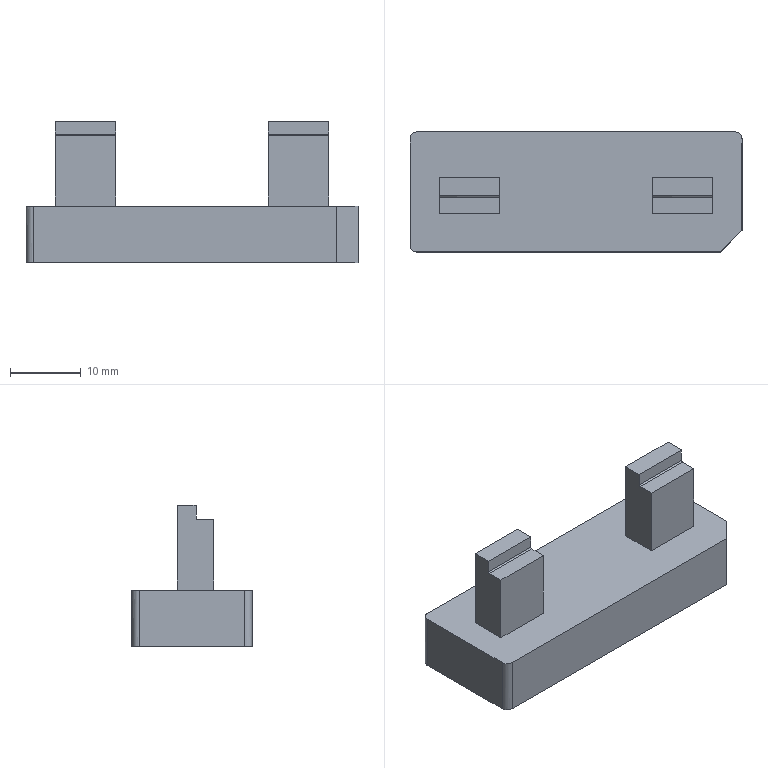NC program | PowerMill | posted by the shop | part box 47 x 17 x 19.985 mm
Lines 1 to 1597 of 62704:
%
G40 G49 G17 G80
( TOOL ID   D10C_1_1_1 )
( TOOL DIA. 10. TIP RAD 0 LENGTH 75.44 )
( Z = -.065 )
T1 M6
T2
G91 G28 Z0
G0 G90 G54
M08
S8000 M3
G0 X0 Y0 M8
G43 Z10.2 H1
X31.28 Y11.28
Z1.135
G1 Z-.065 F6000
X26.28 F10000
X-26.28
Y5.64
X26.28
Y0
X-26.28
Y-5.64
X26.28
Y-11.28
X-26.28
X-31.28
G0 Z10.2
X0 Y0
Z9.885
X-32.38 Y-5.333
Z.691
G1 Z-.509 F6000
X-31.853 F10000
G3 X-27.105 Y-.585 I0 J4.747
G1 Y10.28
G2 X-26.105 Y11.28 I1. J0
G1 X26.105
G2 X27.105 Y10.28 I0 J-1.
G1 Y2.243
X24.596 Y2.127
X24.605 Y1.934
Y-.387
X24.574 Y-1.16
X24.43 Y-1.934
X24.16 Y-2.707
X23.976 Y-3.084
X23.74 Y-3.48
X23.203 Y-4.168
X22.429 Y-4.856
X22.178 Y-5.027
X21.656 Y-5.322
X20.883 Y-5.63
X20.144 Y-5.801
X19.336 Y-5.865
X10.828
X10.055 Y-5.808
X9.281 Y-5.634
X8.508 Y-5.329
X7.972 Y-5.027
X7.734 Y-4.866
X7.028 Y-4.254
X6.41 Y-3.48
X6.187 Y-3.109
X6.165 Y-3.063
X.373 Y-4.753
X.381 Y-4.793
X.384 Y-4.833
G2 X-.192 Y-4.833 I-.288 J0
X.373 Y-4.753 I.288 J0
G1 X6.165 Y-3.063
X5.99 Y-2.707
X5.72 Y-1.934
X5.576 Y-1.16
X5.545 Y-.387
Y1.934
X5.581 Y2.707
X5.731 Y3.48
X.004 Y5.269
X.002 Y5.263
X0 Y5.258
X-.007 Y5.28
X.007
X.005 Y5.274
X.004 Y5.269
X5.731 Y3.48
X6.008 Y4.254
X6.187 Y4.616
X6.436 Y5.027
X6.961 Y5.69
X7.734 Y6.373
X8.034 Y6.574
X8.508 Y6.837
X9.281 Y7.142
X10.055 Y7.316
X10.828 Y7.372
X19.336
X20.109 Y7.314
X20.883 Y7.137
X21.656 Y6.83
X22.116 Y6.574
X22.429 Y6.363
X23.083 Y5.801
X23.714 Y5.027
X23.976 Y4.591
X24.142 Y4.254
X24.419 Y3.48
X24.569 Y2.707
X24.596 Y2.127
X27.105 Y2.243
Y-10.28
G2 X26.105 Y-11.28 I-1. J0
G1 X-26.105
G2 X-27.105 Y-10.28 I0 J1.
G1 Y-.585
X-24.601 Y-.483
X-24.605 Y-.387
Y1.934
X-24.569 Y2.707
X-24.419 Y3.48
X-24.142 Y4.254
X-23.976 Y4.592
X-23.714 Y5.027
X-23.203 Y5.676
X-22.429 Y6.364
X-22.117 Y6.574
X-21.656 Y6.83
X-20.883 Y7.138
X-20.109 Y7.314
X-19.336 Y7.373
X-10.828
X-10.055 Y7.316
X-9.281 Y7.142
X-8.508 Y6.837
X-8.033 Y6.574
X-7.734 Y6.374
X-7.066 Y5.801
X-6.436 Y5.027
X-6.187 Y4.617
X-6.008 Y4.254
X-5.731 Y3.48
X-5.581 Y2.707
X-5.545 Y1.934
Y-.387
X-5.577 Y-1.16
X-5.72 Y-1.934
X-5.99 Y-2.707
X-6.187 Y-3.108
X-6.41 Y-3.48
X-6.961 Y-4.182
X-7.734 Y-4.865
X-7.972 Y-5.027
X-8.508 Y-5.329
X-9.281 Y-5.634
X-10.008 Y-5.801
X-10.828 Y-5.864
X-19.336
X-20.109 Y-5.806
X-20.883 Y-5.629
X-21.656 Y-5.322
X-22.178 Y-5.027
X-22.429 Y-4.855
X-23.121 Y-4.254
X-23.74 Y-3.48
X-23.976 Y-3.083
X-24.159 Y-2.707
X-24.43 Y-1.934
X-24.573 Y-1.16
X-24.601 Y-.483
X-27.105 Y-.585
G0 Z3.297
G1 X-32.38 Y-5.333
G0 Z.297
G1 Z-.903 F6000
X-31.853 F10000
G3 X-27.105 Y-.585 I0 J4.747
G1 X-24.601 Y-.483
X-24.605 Y-.387
Y1.934
X-24.569 Y2.707
X-24.419 Y3.48
X-24.142 Y4.254
X-23.976 Y4.592
X-23.714 Y5.027
X-23.203 Y5.676
X-22.429 Y6.364
X-22.117 Y6.574
X-21.656 Y6.83
X-20.883 Y7.138
X-20.109 Y7.314
X-19.336 Y7.373
X-10.828
X-10.055 Y7.316
X-9.281 Y7.142
X-8.508 Y6.837
X-8.033 Y6.574
X-7.734 Y6.374
X-7.066 Y5.801
X-6.436 Y5.027
X-6.187 Y4.617
X-6.008 Y4.254
X-5.731 Y3.48
X-5.581 Y2.707
X-5.545 Y1.934
Y-.387
X-5.577 Y-1.16
X-5.72 Y-1.934
X-5.99 Y-2.707
X-6.187 Y-3.108
X-6.41 Y-3.48
X-6.961 Y-4.182
X-7.734 Y-4.865
X-7.972 Y-5.027
X-8.508 Y-5.329
X-9.281 Y-5.634
X-10.008 Y-5.801
X-10.828 Y-5.864
X-19.336
X-20.109 Y-5.806
X-20.883 Y-5.629
X-21.656 Y-5.322
X-22.178 Y-5.027
X-22.429 Y-4.855
X-23.121 Y-4.254
X-23.74 Y-3.48
X-23.976 Y-3.083
X-24.159 Y-2.707
X-24.43 Y-1.934
X-24.573 Y-1.16
X-24.601 Y-.483
X-27.105 Y-.585
Y10.28
G2 X-26.105 Y11.28 I1. J0
G1 X26.105
G2 X27.105 Y10.28 I0 J-1.
G1 Y2.243
X24.596 Y2.127
X24.605 Y1.934
Y-.387
X24.574 Y-1.16
X24.43 Y-1.934
X24.16 Y-2.707
X23.976 Y-3.084
X23.74 Y-3.48
X23.203 Y-4.168
X22.429 Y-4.856
X22.178 Y-5.027
X21.656 Y-5.322
X20.883 Y-5.63
X20.144 Y-5.801
X19.336 Y-5.865
X10.828
X10.055 Y-5.808
X9.281 Y-5.634
X8.508 Y-5.329
X7.972 Y-5.027
X7.734 Y-4.866
X7.028 Y-4.254
X6.41 Y-3.48
X6.187 Y-3.109
X6.165 Y-3.063
X.373 Y-4.753
X.381 Y-4.793
X.384 Y-4.833
G2 X-.192 Y-4.833 I-.288 J0
X.373 Y-4.753 I.288 J0
G1 X6.165 Y-3.063
X5.99 Y-2.707
X5.72 Y-1.934
X5.576 Y-1.16
X5.545 Y-.387
Y1.934
X5.581 Y2.707
X5.731 Y3.48
X.004 Y5.269
X.002 Y5.263
X0 Y5.258
X-.007 Y5.28
X.007
X.005 Y5.274
X.004 Y5.269
X5.731 Y3.48
X6.008 Y4.254
X6.187 Y4.616
X6.436 Y5.027
X6.961 Y5.69
X7.734 Y6.373
X8.034 Y6.574
X8.508 Y6.837
X9.281 Y7.142
X10.055 Y7.316
X10.828 Y7.372
X19.336
X20.109 Y7.314
X20.883 Y7.137
X21.656 Y6.83
X22.116 Y6.574
X22.429 Y6.363
X23.083 Y5.801
X23.714 Y5.027
X23.976 Y4.591
X24.142 Y4.254
X24.419 Y3.48
X24.569 Y2.707
X24.596 Y2.127
X27.105 Y2.243
Y-10.28
G2 X26.105 Y-11.28 I-1. J0
G1 X-26.105
G2 X-27.105 Y-10.28 I0 J1.
G1 Y-.585
G0 Z2.903
G1 X-32.38 Y-5.333
G0 Z-.097
G1 Z-1.297 F6000
X-31.853 F10000
G3 X-27.105 Y-.585 I0 J4.747
G1 X-24.601 Y-.483
X-24.605 Y-.387
Y1.934
X-24.569 Y2.707
X-24.419 Y3.48
X-24.142 Y4.254
X-23.976 Y4.592
X-23.714 Y5.027
X-23.203 Y5.676
X-22.429 Y6.364
X-22.117 Y6.574
X-21.656 Y6.83
X-20.883 Y7.138
X-20.109 Y7.314
X-19.336 Y7.373
X-10.828
X-10.055 Y7.316
X-9.281 Y7.142
X-8.508 Y6.837
X-8.033 Y6.574
X-7.734 Y6.374
X-7.066 Y5.801
X-6.436 Y5.027
X-6.187 Y4.617
X-6.008 Y4.254
X-5.731 Y3.48
X-5.581 Y2.707
X-5.545 Y1.934
Y-.387
X-5.577 Y-1.16
X-5.72 Y-1.934
X-5.99 Y-2.707
X-6.187 Y-3.108
X-6.41 Y-3.48
X-6.961 Y-4.182
X-7.734 Y-4.865
X-7.972 Y-5.027
X-8.508 Y-5.329
X-9.281 Y-5.634
X-10.008 Y-5.801
X-10.828 Y-5.864
X-19.336
X-20.109 Y-5.806
X-20.883 Y-5.629
X-21.656 Y-5.322
X-22.178 Y-5.027
X-22.429 Y-4.855
X-23.121 Y-4.254
X-23.74 Y-3.48
X-23.976 Y-3.083
X-24.16 Y-2.707
X-24.43 Y-1.934
X-24.573 Y-1.16
X-24.601 Y-.483
X-27.105 Y-.585
Y10.28
G2 X-26.105 Y11.28 I1. J0
G1 X26.105
G2 X27.105 Y10.28 I0 J-1.
G1 Y2.243
X24.596 Y2.127
X24.605 Y1.934
Y-.387
X24.574 Y-1.16
X24.43 Y-1.934
X24.16 Y-2.707
X23.976 Y-3.084
X23.74 Y-3.48
X23.203 Y-4.168
X22.429 Y-4.856
X22.178 Y-5.027
X21.656 Y-5.322
X20.883 Y-5.63
X20.144 Y-5.801
X19.336 Y-5.865
X10.828
X10.055 Y-5.808
X9.281 Y-5.634
X8.508 Y-5.329
X7.972 Y-5.027
X7.734 Y-4.866
X7.028 Y-4.254
X6.41 Y-3.48
X6.187 Y-3.109
X6.165 Y-3.063
X.373 Y-4.753
X.381 Y-4.793
X.384 Y-4.833
G2 X-.192 Y-4.833 I-.288 J0
X.373 Y-4.753 I.288 J0
G1 X6.165 Y-3.063
X5.99 Y-2.707
X5.72 Y-1.934
X5.576 Y-1.16
X5.545 Y-.387
Y1.934
X5.581 Y2.707
X5.731 Y3.48
X.004 Y5.269
X.002 Y5.263
X0 Y5.258
X-.007 Y5.28
X.007
X.005 Y5.274
X.004 Y5.269
X5.731 Y3.48
X6.008 Y4.254
X6.187 Y4.616
X6.436 Y5.027
X6.961 Y5.69
X7.734 Y6.373
X8.034 Y6.574
X8.508 Y6.837
X9.281 Y7.142
X10.055 Y7.316
X10.828 Y7.372
X19.336
X20.109 Y7.314
X20.883 Y7.137
X21.656 Y6.83
X22.116 Y6.574
X22.429 Y6.363
X23.083 Y5.801
X23.714 Y5.027
X23.976 Y4.591
X24.142 Y4.254
X24.419 Y3.48
X24.569 Y2.707
X24.596 Y2.127
X27.105 Y2.243
Y-10.28
G2 X26.105 Y-11.28 I-1. J0
G1 X-26.105
G2 X-27.105 Y-10.28 I0 J1.
G1 Y-.585
G0 Z2.509
G1 X-32.38 Y-5.333
G0 Z-.491
G1 Z-1.691 F6000
X-31.853 F10000
G3 X-27.105 Y-.585 I0 J4.747
G1 X-24.601 Y-.483
X-24.605 Y-.387
Y1.934
X-24.569 Y2.707
X-24.419 Y3.48
X-24.142 Y4.254
X-23.976 Y4.592
X-23.714 Y5.027
X-23.203 Y5.676
X-22.429 Y6.364
X-22.117 Y6.574
X-21.656 Y6.83
X-20.883 Y7.138
X-20.109 Y7.314
X-19.336 Y7.373
X-10.828
X-10.055 Y7.316
X-9.281 Y7.142
X-8.508 Y6.837
X-8.033 Y6.574
X-7.734 Y6.374
X-7.066 Y5.801
X-6.436 Y5.027
X-6.187 Y4.617
X-6.008 Y4.254
X-5.731 Y3.48
X-5.581 Y2.707
X-5.545 Y1.934
Y-.387
X-5.576 Y-1.16
X-5.72 Y-1.934
X-5.99 Y-2.707
X-6.187 Y-3.108
X-6.41 Y-3.48
X-6.961 Y-4.182
X-7.734 Y-4.865
X-7.972 Y-5.027
X-8.508 Y-5.329
X-9.281 Y-5.634
X-10.008 Y-5.801
X-10.828 Y-5.864
X-19.336
X-20.109 Y-5.806
X-20.883 Y-5.629
X-21.656 Y-5.322
X-22.178 Y-5.027
X-22.429 Y-4.855
X-23.121 Y-4.254
X-23.74 Y-3.48
X-23.976 Y-3.083
X-24.16 Y-2.707
X-24.43 Y-1.934
X-24.574 Y-1.16
X-24.601 Y-.483
X-27.105 Y-.585
Y10.28
G2 X-26.105 Y11.28 I1. J0
G1 X26.105
G2 X27.105 Y10.28 I0 J-1.
G1 Y2.243
X24.596 Y2.127
X24.605 Y1.934
Y-.387
X24.574 Y-1.16
X24.43 Y-1.934
X24.16 Y-2.707
X23.976 Y-3.084
X23.74 Y-3.48
X23.203 Y-4.168
X22.429 Y-4.856
X22.178 Y-5.027
X21.656 Y-5.322
X20.883 Y-5.63
X20.144 Y-5.801
X19.336 Y-5.865
X10.828
X10.055 Y-5.808
X9.281 Y-5.634
X8.508 Y-5.329
X7.972 Y-5.027
X7.734 Y-4.866
X7.028 Y-4.254
X6.41 Y-3.48
X6.187 Y-3.109
X6.165 Y-3.063
X.373 Y-4.753
X.381 Y-4.793
X.384 Y-4.833
G2 X-.192 Y-4.833 I-.288 J0
X.373 Y-4.753 I.288 J0
G1 X6.165 Y-3.063
X5.99 Y-2.707
X5.72 Y-1.934
X5.576 Y-1.16
X5.545 Y-.387
Y1.934
X5.581 Y2.707
X5.731 Y3.48
X.004 Y5.269
X.002 Y5.263
X0 Y5.258
X-.007 Y5.28
X.007
X.005 Y5.274
X.004 Y5.269
X5.731 Y3.48
X6.008 Y4.254
X6.187 Y4.616
X6.436 Y5.027
X6.961 Y5.69
X7.734 Y6.373
X8.034 Y6.574
X8.508 Y6.837
X9.281 Y7.142
X10.055 Y7.316
X10.828 Y7.372
X19.336
X20.109 Y7.314
X20.883 Y7.137
X21.656 Y6.83
X22.116 Y6.574
X22.429 Y6.363
X23.083 Y5.801
X23.714 Y5.027
X23.976 Y4.591
X24.142 Y4.254
X24.419 Y3.48
X24.569 Y2.707
X24.596 Y2.127
X27.105 Y2.243
Y-10.28
G2 X26.105 Y-11.28 I-1. J0
G1 X-26.105
G2 X-27.105 Y-10.28 I0 J1.
G1 Y-.585
G0 Z2.115
G1 X-32.38 Y-5.333
G0 Z-.885
G1 Z-2.085 F6000
X-31.853 F10000
G3 X-27.105 Y-.585 I0 J4.747
G1 Y-.387
X-24.605
Y1.934
X-24.569 Y2.707
X-24.419 Y3.48
X-24.142 Y4.254
X-23.976 Y4.592
X-23.714 Y5.027
X-23.203 Y5.676
X-22.429 Y6.364
X-22.117 Y6.574
X-21.656 Y6.83
X-20.883 Y7.138
X-20.109 Y7.314
X-19.336 Y7.373
X-10.828
X-10.055 Y7.316
X-9.281 Y7.142
X-8.508 Y6.837
X-8.033 Y6.574
X-7.734 Y6.374
X-7.066 Y5.801
X-6.436 Y5.027
X-6.187 Y4.617
X-6.008 Y4.254
X-5.731 Y3.48
X-5.581 Y2.707
X-5.545 Y1.934
Y-.387
X-5.573 Y-1.16
X-5.688 Y-1.934
X-5.976 Y-2.707
X-6.187 Y-3.145
X-6.384 Y-3.48
X-6.961 Y-4.224
X-7.734 Y-4.91
X-8.508 Y-5.376
X-9.281 Y-5.683
X-9.738 Y-5.801
X-10.055 Y-5.858
X-10.828 Y-5.914
X-19.336
X-20.109 Y-5.855
X-20.883 Y-5.679
X-21.656 Y-5.37
X-22.429 Y-4.901
X-23.164 Y-4.254
X-23.775 Y-3.48
X-24.175 Y-2.707
X-24.438 Y-1.934
X-24.58 Y-1.16
X-24.605 Y-.387
X-27.105
Y10.28
G2 X-26.105 Y11.28 I1. J0
G1 X26.105
G2 X27.105 Y10.28 I0 J-1.
G1 Y2.243
X24.596 Y2.127
X24.605 Y1.934
Y-.387
X24.58 Y-1.16
X24.438 Y-1.934
X24.175 Y-2.707
X23.976 Y-3.122
X23.764 Y-3.48
X23.203 Y-4.21
X22.429 Y-4.901
X22.254 Y-5.027
X21.656 Y-5.37
X20.883 Y-5.679
X20.423 Y-5.801
X20.109 Y-5.856
X19.336 Y-5.915
X10.828
X10.055 Y-5.859
X9.281 Y-5.683
X8.508 Y-5.377
X7.896 Y-5.027
X7.734 Y-4.911
X6.986 Y-4.254
X6.384 Y-3.48
X6.187 Y-3.146
X6.154 Y-3.078
X.315 Y-4.781
X.322 Y-4.816
X.325 Y-4.851
G2 X-.18 Y-4.851 I-.252 J0
X.315 Y-4.781 I.252 J0
G1 X6.154 Y-3.078
X5.97 Y-2.707
X5.688 Y-1.934
X5.573 Y-1.16
X5.545 Y-.387
Y1.934
X5.581 Y2.707
X5.731 Y3.48
X.004 Y5.269
X.002 Y5.263
X0 Y5.258
X-.007 Y5.28
X.007
X.005 Y5.274
X.004 Y5.269
X5.731 Y3.48
X6.008 Y4.254
X6.187 Y4.616
X6.436 Y5.027
X6.961 Y5.69
X7.734 Y6.373
X8.034 Y6.574
X8.508 Y6.837
X9.281 Y7.142
X10.055 Y7.316
X10.828 Y7.372
X19.336
X20.109 Y7.314
X20.883 Y7.137
X21.656 Y6.83
X22.116 Y6.574
X22.429 Y6.363
X23.084 Y5.801
X23.714 Y5.027
X23.976 Y4.591
X24.142 Y4.254
X24.419 Y3.48
X24.569 Y2.707
X24.596 Y2.127
X27.105 Y2.243
Y-10.28
G2 X26.105 Y-11.28 I-1. J0
G1 X-26.105
G2 X-27.105 Y-10.28 I0 J1.
G1 Y-.585
G0 Z1.719
G1 X-32.38 Y-5.333
G0 Z-1.281
G1 Z-2.481 F6000
X-31.853 F10000
G3 X-27.105 Y-.585 I0 J4.747
G1 Y10.28
G2 X-26.105 Y11.28 I1. J0
G1 X26.105
G2 X27.105 Y10.28 I0 J-1.
G1 Y2.243
X24.596 Y2.127
X24.605 Y1.934
Y1.913
Y-.387
X24.598 Y-.592
X24.591 Y-3.48
X24.476 Y-4.254
X24.238 Y-5.027
X23.857 Y-5.801
X23.294 Y-6.574
X22.451 Y-7.348
X21.656 Y-7.83
X20.935 Y-8.121
X20.109 Y-8.314
X19.336 Y-8.372
X10.828
X10.055 Y-8.316
X9.281 Y-8.142
X8.508 Y-7.837
X7.734 Y-7.373
X6.961 Y-6.69
X6.293 Y-5.801
X5.912 Y-5.027
X5.674 Y-4.254
X5.559 Y-3.48
X5.552 Y-.571
X5.549 Y-.497
X.081
Y-3.098
G3 X.275 Y-5.117 I10.557 J0
G1 X.325 Y-5.369
X.375 Y-5.597
G2 X.2 Y-5.815 I-.175 J-.039
G1 X-.2
G2 X-.375 Y-5.597 I0 J.179
G1 X-.348 Y-5.473
G3 X-.027 Y-2.387 I-13.16 J2.925
G1 X-.082 Y2.241
G3 X-.358 Y4.506 I-10.471 J-.124
G1 X-.401 Y4.69
X-.511 Y5.097
X-.646 Y5.497
X-.681 Y5.589
G2 X-.525 Y5.815 I.156 J.059
G1 X.525
G2 X.681 Y5.589 I0 J-.167
G1 X.647 Y5.497
X.512 Y5.101
X.403 Y4.696
X.362 Y4.522
G3 X.081 Y2.104 I10.268 J-2.418
G1 Y-.497
X5.549
X5.545 Y-.387
Y1.914
Y1.934
X5.581 Y2.707
X5.731 Y3.48
X6.008 Y4.254
X6.187 Y4.616
X6.436 Y5.027
X6.961 Y5.69
X7.734 Y6.373
X8.034 Y6.574
X8.508 Y6.837
X9.281 Y7.142
X10.055 Y7.316
X10.828 Y7.372
X19.336
X20.109 Y7.314
X20.883 Y7.137
X21.656 Y6.83
X22.116 Y6.574
X22.429 Y6.363
X23.084 Y5.801
X23.714 Y5.027
X23.976 Y4.591
X24.142 Y4.254
X24.419 Y3.48
X24.569 Y2.707
X24.596 Y2.127
X27.105 Y2.243
Y-10.28
G2 X26.105 Y-11.28 I-1. J0
G1 X-26.105
G2 X-27.105 Y-10.28 I0 J1.
G1 Y-3.487
X-24.591 Y-3.48
X-24.598 Y-.591
X-24.605 Y-.387
Y1.913
Y1.934
X-24.569 Y2.707
X-24.419 Y3.48
X-24.142 Y4.254
X-23.976 Y4.592
X-23.714 Y5.027
X-23.203 Y5.676
X-22.429 Y6.364
X-22.117 Y6.574
X-21.656 Y6.83
X-20.883 Y7.138
X-20.109 Y7.314
X-19.336 Y7.373
X-10.828
X-10.055 Y7.316
X-9.281 Y7.142
X-8.508 Y6.837
X-8.033 Y6.574
X-7.734 Y6.374
X-7.066 Y5.801
X-6.436 Y5.027
X-6.187 Y4.617
X-6.008 Y4.254
X-5.731 Y3.48
X-5.581 Y2.707
X-5.545 Y1.934
Y1.914
Y-.387
X-5.552 Y-.571
X-5.559 Y-3.48
X-5.674 Y-4.254
X-5.912 Y-5.027
X-6.293 Y-5.801
X-6.856 Y-6.574
X-7.7 Y-7.348
X-8.508 Y-7.836
X-9.216 Y-8.121
X-10.055 Y-8.315
X-10.828 Y-8.372
X-19.336
X-20.109 Y-8.313
X-20.883 Y-8.137
X-21.656 Y-7.83
X-22.45 Y-7.348
X-23.203 Y-6.675
X-23.857 Y-5.801
X-24.238 Y-5.027
X-24.476 Y-4.254
X-24.591 Y-3.48
X-27.105 Y-3.487
Y-.585
G0 Z1.322
G1 X-32.38 Y-5.333
G0 Z-1.678
G1 Z-2.878 F6000
X-31.853 F10000
G3 X-27.105 Y-.585 I0 J4.747
G1 Y10.28
G2 X-26.105 Y11.28 I1. J0
G1 X26.105
G2 X27.105 Y10.28 I0 J-1.
G1 Y2.243
X24.596 Y2.127
X24.605 Y1.934
Y1.894
Y-.387
X24.598 Y-.59
X24.591 Y-3.48
X24.476 Y-4.254
X24.238 Y-5.027
X23.857 Y-5.801
X23.294 Y-6.574
X22.451 Y-7.348
X21.656 Y-7.83
X20.935 Y-8.121
X20.109 Y-8.314
X19.336 Y-8.372
X10.828
X10.055 Y-8.316
X9.281 Y-8.142
X8.508 Y-7.837
X7.734 Y-7.373
X6.961 Y-6.69
X6.293 Y-5.801
X5.912 Y-5.027
X5.674 Y-4.254
X5.559 Y-3.48
X5.552 Y-.569
X5.549 Y-.497
X.081
Y-3.098
G3 X.276 Y-5.12 I10.562 J0
G1 X.325 Y-5.37
X.375 Y-5.597
G2 X.2 Y-5.815 I-.175 J-.039
G1 X-.2
G2 X-.375 Y-5.597 I0 J.179
G1 X-.347 Y-5.472
G3 X-.027 Y-2.383 I-13.169 J2.926
G1 X-.083 Y2.254
G3 X-.355 Y4.494 I-10.396 J-.126
G1 X-.4 Y4.685
X-.51 Y5.095
X-.646 Y5.497
X-.681 Y5.589
G2 X-.524 Y5.815 I.157 J.059
G1 X.525
G2 X.681 Y5.589 I0 J-.167
G1 X.647 Y5.497
X.512 Y5.101
X.403 Y4.698
X.362 Y4.525
G3 X.081 Y2.103 I10.273 J-2.421
G1 Y-.497
X5.549
X5.545 Y-.387
Y1.893
Y1.934
X5.581 Y2.707
X5.731 Y3.48
X6.008 Y4.254
X6.187 Y4.616
X6.436 Y5.027
X6.961 Y5.69
X7.734 Y6.373
X8.034 Y6.574
X8.508 Y6.837
X9.281 Y7.142
X10.055 Y7.316
X10.828 Y7.372
X19.336
X20.109 Y7.314
X20.883 Y7.137
X21.656 Y6.83
X22.116 Y6.574
X22.429 Y6.363
X23.084 Y5.801
X23.714 Y5.027
X23.976 Y4.591
X24.142 Y4.254
X24.419 Y3.48
X24.569 Y2.707
X24.596 Y2.127
X27.105 Y2.243
Y-10.28
G2 X26.105 Y-11.28 I-1. J0
G1 X-26.105
G2 X-27.105 Y-10.28 I0 J1.
G1 Y-3.487
X-24.591 Y-3.48
X-24.598 Y-.589
X-24.605 Y-.387
Y1.894
Y1.934
X-24.569 Y2.707
X-24.419 Y3.48
X-24.142 Y4.254
X-23.976 Y4.592
X-23.714 Y5.027
X-23.203 Y5.676
X-22.429 Y6.364
X-22.117 Y6.574
X-21.656 Y6.83
X-20.883 Y7.138
X-20.109 Y7.314
X-19.336 Y7.373
X-10.828
X-10.055 Y7.316
X-9.281 Y7.142
X-8.508 Y6.837
X-8.033 Y6.574
X-7.734 Y6.374
X-7.066 Y5.801
X-6.436 Y5.027
X-6.187 Y4.617
X-6.008 Y4.254
X-5.731 Y3.48
X-5.581 Y2.707
X-5.545 Y1.934
Y1.893
Y-.387
X-5.552 Y-.569
X-5.559 Y-3.48
X-5.674 Y-4.254
X-5.912 Y-5.027
X-6.293 Y-5.801
X-6.856 Y-6.574
X-7.7 Y-7.348
X-8.508 Y-7.836
X-9.216 Y-8.121
X-10.055 Y-8.315
X-10.828 Y-8.372
X-19.336
X-20.109 Y-8.313
X-20.883 Y-8.137
X-21.656 Y-7.83
X-22.45 Y-7.348
X-23.203 Y-6.675
X-23.857 Y-5.801
X-24.238 Y-5.027
X-24.476 Y-4.254
X-24.591 Y-3.48
X-27.105 Y-3.487
Y-.585
G0 Z.926
G1 X-32.38 Y-5.333
G0 Z-2.074
G1 Z-3.274 F6000
X-31.853 F10000
G3 X-27.105 Y-.585 I0 J4.747
G1 Y10.28
G2 X-26.105 Y11.28 I1. J0
G1 X26.105
G2 X27.105 Y10.28 I0 J-1.
G1 Y2.243
X24.596 Y2.127
X24.605 Y1.934
Y1.873
Y-.387
X24.598 Y-.588
X24.591 Y-3.48
X24.476 Y-4.254
X24.238 Y-5.027
X23.857 Y-5.801
X23.294 Y-6.574
X22.451 Y-7.348
X21.656 Y-7.83
X20.935 Y-8.121
X20.109 Y-8.314
X19.336 Y-8.372
X10.828
X10.055 Y-8.316
X9.281 Y-8.142
X8.508 Y-7.837
X7.734 Y-7.373
X6.961 Y-6.69
X6.293 Y-5.801
X5.912 Y-5.027
X5.674 Y-4.254
X5.559 Y-3.48
X5.552 Y-.568
X5.549 Y-.497
X.081
Y-3.097
G3 X.277 Y-5.123 I10.568 J0
G1 X.325 Y-5.37
X.375 Y-5.597
G2 X.2 Y-5.815 I-.175 J-.039
G1 X-.2
G2 X-.375 Y-5.597 I0 J.18
G1 X-.347 Y-5.471
G3 X-.027 Y-2.378 I-13.178 J2.927
G1 X-.084 Y2.266
G3 X-.353 Y4.483 I-10.328 J-.127
G1 X-.399 Y4.681
X-.509 Y5.093
X-.646 Y5.497
X-.681 Y5.589
G2 X-.524 Y5.815 I.157 J.059
G1 X.524
G2 X.681 Y5.589 I0 J-.167
G1 X.646 Y5.497
X.512 Y5.102
X.403 Y4.699
X.363 Y4.527
G3 X.081 Y2.103 I10.278 J-2.425
G1 Y-.497
X5.549
X5.545 Y-.387
Y1.873
Y1.934
X5.581 Y2.707
X5.731 Y3.48
X6.008 Y4.254
X6.187 Y4.616
X6.436 Y5.027
X6.961 Y5.69
X7.734 Y6.373
X8.034 Y6.574
X8.508 Y6.837
X9.281 Y7.142
X10.055 Y7.316
X10.828 Y7.372
X19.336
X20.109 Y7.314
X20.883 Y7.137
X21.656 Y6.83
X22.116 Y6.574
X22.429 Y6.363
X23.084 Y5.801
X23.714 Y5.027
X23.976 Y4.591
X24.142 Y4.254
X24.419 Y3.48
X24.569 Y2.707
X24.596 Y2.127
X27.105 Y2.243
Y-10.28
G2 X26.105 Y-11.28 I-1. J0
G1 X-26.105
G2 X-27.105 Y-10.28 I0 J1.
G1 Y-3.487
X-24.591 Y-3.48
X-24.598 Y-.587
X-24.605 Y-.387
Y1.873
Y1.934
X-24.569 Y2.707
X-24.419 Y3.48
X-24.142 Y4.254
X-23.976 Y4.592
X-23.714 Y5.027
X-23.203 Y5.676
X-22.429 Y6.364
X-22.117 Y6.574
X-21.656 Y6.83
X-20.883 Y7.138
X-20.109 Y7.314
X-19.336 Y7.373
X-10.828
X-10.055 Y7.316
X-9.281 Y7.142
X-8.508 Y6.837
X-8.033 Y6.574
X-7.734 Y6.374
X-7.066 Y5.801
X-6.436 Y5.027
X-6.187 Y4.617
X-6.008 Y4.254
X-5.731 Y3.48
X-5.581 Y2.707
X-5.545 Y1.934
Y1.873
Y-.387
X-5.552 Y-.568
X-5.559 Y-3.48
X-5.674 Y-4.254
X-5.912 Y-5.027
X-6.293 Y-5.801
X-6.856 Y-6.574
X-7.7 Y-7.348
X-8.508 Y-7.836
X-9.216 Y-8.121
X-10.055 Y-8.315
X-10.828 Y-8.372
X-19.336
X-20.109 Y-8.313
X-20.883 Y-8.137
X-21.656 Y-7.83
X-22.45 Y-7.348
X-23.203 Y-6.675
X-23.857 Y-5.801
X-24.238 Y-5.027
X-24.476 Y-4.254
X-24.591 Y-3.48
X-27.105 Y-3.487
Y-.585
G0 Z.53
G1 X-32.38 Y-5.333
G0 Z-2.47
G1 Z-3.67 F6000
X-31.853 F10000
G3 X-27.105 Y-.585 I0 J4.747
G1 Y10.28
G2 X-26.105 Y11.28 I1. J0
G1 X26.105
G2 X27.105 Y10.28 I0 J-1.
G1 Y2.243
X24.596 Y2.127
X24.605 Y1.934
Y1.853
Y-.387
X24.598 Y-.587
X24.591 Y-3.48
X24.476 Y-4.254
X24.238 Y-5.027
X23.857 Y-5.801
X23.294 Y-6.574
X22.451 Y-7.348
X21.656 Y-7.83
X20.935 Y-8.121
X20.109 Y-8.314
X19.336 Y-8.372
X10.828
X10.055 Y-8.316
X9.281 Y-8.142
X8.508 Y-7.837
X7.734 Y-7.373
X6.961 Y-6.69
X6.293 Y-5.801
X5.912 Y-5.027
X5.674 Y-4.254
X5.559 Y-3.48
X5.552 Y-.566
X5.549 Y-.497
X.081 Y-.498
Y-3.097
G3 X.277 Y-5.126 I10.574 J0
G1 X.325 Y-5.371
X.375 Y-5.596
G2 X.2 Y-5.815 I-.176 J-.039
G1 X-.2
G2 X-.375 Y-5.596 I0 J.18
G1 X-.347 Y-5.47
G3 X-.027 Y-2.374 I-13.187 J2.928
G1 X-.085 Y2.277
G3 X-.351 Y4.473 I-10.264 J-.128
G1 X-.398 Y4.678
X-.509 Y5.091
X-.646 Y5.497
X-.681 Y5.588
G2 X-.524 Y5.815 I.157 J.059
G1 X.524
G2 X.681 Y5.588 I0 J-.168
G1 X.646 Y5.497
X.512 Y5.102
X.404 Y4.7
X.363 Y4.53
G3 X.081 Y2.102 I10.283 J-2.428
G1 Y-.498
X5.549 Y-.497
X5.545 Y-.387
Y1.853
Y1.934
X5.581 Y2.707
X5.731 Y3.48
X6.008 Y4.254
X6.187 Y4.616
X6.436 Y5.027
X6.961 Y5.69
X7.734 Y6.373
X8.034 Y6.574
X8.508 Y6.837
X9.281 Y7.142
X10.055 Y7.316
X10.828 Y7.372
X19.336
X20.109 Y7.314
X20.883 Y7.137
X21.656 Y6.83
X22.116 Y6.574
X22.429 Y6.363
X23.084 Y5.801
X23.714 Y5.027
X23.976 Y4.591
X24.142 Y4.254
X24.419 Y3.48
X24.569 Y2.707
X24.596 Y2.127
X27.105 Y2.243
Y-10.28
G2 X26.105 Y-11.28 I-1. J0
G1 X-26.105
G2 X-27.105 Y-10.28 I0 J1.
G1 Y-3.487
X-24.591 Y-3.48
X-24.598 Y-.586
X-24.605 Y-.387
Y1.853
Y1.934
X-24.569 Y2.707
X-24.419 Y3.48
X-24.142 Y4.254
X-23.976 Y4.592
X-23.714 Y5.027
X-23.203 Y5.676
X-22.429 Y6.364
X-22.117 Y6.574
X-21.656 Y6.83
X-20.883 Y7.138
X-20.109 Y7.314
X-19.336 Y7.373
X-10.828
X-10.055 Y7.316
X-9.281 Y7.142
X-8.508 Y6.837
X-8.033 Y6.574
X-7.734 Y6.374
X-7.066 Y5.801
X-6.436 Y5.027
X-6.187 Y4.617
X-6.008 Y4.254
X-5.731 Y3.48
X-5.581 Y2.707
X-5.545 Y1.934
Y1.853
Y-.387
X-5.552 Y-.566
X-5.559 Y-3.48
X-5.674 Y-4.254
X-5.912 Y-5.027
X-6.293 Y-5.801
X-6.856 Y-6.574
X-7.7 Y-7.348
X-8.508 Y-7.836
X-9.216 Y-8.121
X-10.055 Y-8.315
X-10.828 Y-8.372
X-19.336
X-20.109 Y-8.313
X-20.883 Y-8.137
X-21.656 Y-7.83
X-22.45 Y-7.348
X-23.203 Y-6.675
X-23.857 Y-5.801
X-24.238 Y-5.027
X-24.476 Y-4.254
X-24.591 Y-3.48
X-27.105 Y-3.487
Y-.585
G0 Z.134
G1 X-32.38 Y-5.333
G0 Z-2.866
G1 Z-4.066 F6000
X-31.853 F10000
G3 X-27.105 Y-.585 I0 J4.747
G1 Y10.28
G2 X-26.105 Y11.28 I1. J0
G1 X26.105
G2 X27.105 Y10.28 I0 J-1.
G1 Y2.243
X24.596 Y2.127
X24.605 Y1.934
Y1.833
Y-.387
X24.598 Y-.585
X24.591 Y-3.48
X24.476 Y-4.254
X24.238 Y-5.027
X23.857 Y-5.801
X23.294 Y-6.574
X22.451 Y-7.348
X21.656 Y-7.83
X20.935 Y-8.121
X20.109 Y-8.314
X19.336 Y-8.372
X10.828
X10.055 Y-8.316
X9.281 Y-8.142
X8.508 Y-7.837
X7.734 Y-7.373
X6.961 Y-6.69
X6.293 Y-5.801
X5.912 Y-5.027
X5.674 Y-4.254
X5.559 Y-3.48
X5.552 Y-.564
X5.549 Y-.498
X.081
Y-3.097
G3 X.278 Y-5.128 I10.579 J0
G1 X.326 Y-5.371
X.375 Y-5.596
G2 X.199 Y-5.815 I-.176 J-.039
G1 X-.199
G2 X-.375 Y-5.596 I0 J.18
G1 X-.347 Y-5.469
G3 X-.027 Y-2.369 I-13.196 J2.929
G1 X-.086 Y2.287
G3 X-.349 Y4.464 I-10.204 J-.129
G1 X-.398 Y4.675
X-.508 Y5.09
X-.646 Y5.496
X-.681 Y5.588
G2 X-.524 Y5.815 I.157 J.059
G1 X.524
G2 X.681 Y5.588 I0 J-.168
G1 X.646 Y5.496
X.512 Y5.103
X.404 Y4.702
X.364 Y4.533
G3 X.081 Y2.101 I10.288 J-2.432
G1 Y-.498
X5.549
X5.545 Y-.387
Y1.833
Y1.934
X5.581 Y2.707
X5.731 Y3.48
X6.008 Y4.254
X6.187 Y4.616
X6.436 Y5.027
X6.961 Y5.69
X7.734 Y6.373
X8.034 Y6.574
X8.508 Y6.837
X9.281 Y7.142
X10.055 Y7.316
X10.828 Y7.372
X19.336
X20.109 Y7.314
X20.883 Y7.137
X21.656 Y6.83
X22.116 Y6.574
X22.429 Y6.363
X23.084 Y5.801
X23.714 Y5.027
X23.976 Y4.591
X24.142 Y4.254
X24.419 Y3.48
X24.569 Y2.707
X24.596 Y2.127
X27.105 Y2.243
Y-10.28
G2 X26.105 Y-11.28 I-1. J0
G1 X-26.105
G2 X-27.105 Y-10.28 I0 J1.
G1 Y-3.487
X-24.591 Y-3.48
X-24.598 Y-.584
X-24.605 Y-.387
Y1.833
Y1.934
X-24.569 Y2.707
X-24.419 Y3.48
X-24.142 Y4.254
X-23.976 Y4.592
X-23.714 Y5.027
X-23.203 Y5.676
X-22.429 Y6.364
X-22.117 Y6.574
X-21.656 Y6.83
X-20.883 Y7.138
X-20.109 Y7.314
X-19.336 Y7.373
X-10.828
X-10.055 Y7.316
X-9.281 Y7.142
X-8.508 Y6.837
X-8.033 Y6.574
X-7.734 Y6.374
X-7.066 Y5.801
X-6.436 Y5.027
X-6.187 Y4.617
X-6.008 Y4.254
X-5.731 Y3.48
X-5.581 Y2.707
X-5.545 Y1.934
Y1.833
Y-.387
X-5.552 Y-.564
X-5.559 Y-3.48
X-5.674 Y-4.254
X-5.912 Y-5.027
X-6.293 Y-5.801
X-6.856 Y-6.574
X-7.7 Y-7.348
X-8.508 Y-7.836
X-9.216 Y-8.121
X-10.055 Y-8.315
X-10.828 Y-8.372
X-19.336
X-20.109 Y-8.313
X-20.883 Y-8.137
X-21.656 Y-7.83
X-22.45 Y-7.348
X-23.203 Y-6.675
X-23.857 Y-5.801
X-24.238 Y-5.027
X-24.476 Y-4.254
X-24.591 Y-3.48
X-27.105 Y-3.487
Y-.585
G0 Z-.262
G1 X-32.38 Y-5.333
G0 Z-3.262
G1 Z-4.462 F6000
X-31.853 F10000
G3 X-27.105 Y-.585 I0 J4.747
G1 Y10.28
G2 X-26.105 Y11.28 I1. J0
G1 X26.105
G2 X27.105 Y10.28 I0 J-1.
G1 Y2.243
X24.596 Y2.127
X24.605 Y1.934
Y1.813
Y-.387
X24.598 Y-.583
X24.591 Y-3.48
X24.476 Y-4.254
X24.238 Y-5.027
X23.857 Y-5.801
X23.294 Y-6.574
X22.451 Y-7.348
X21.656 Y-7.83
X20.935 Y-8.121
X20.109 Y-8.314
X19.336 Y-8.372
X10.828
X10.055 Y-8.316
X9.281 Y-8.142
X8.508 Y-7.837
X7.734 Y-7.373
X6.961 Y-6.69
X6.293 Y-5.801
X5.912 Y-5.027
X5.674 Y-4.254
X5.559 Y-3.48
X5.552 Y-.563
X5.549 Y-.498
X.081
Y-3.096
G3 X.278 Y-5.131 I10.585 J0
G1 X.313 Y-5.308
X.375 Y-5.596
G2 X.199 Y-5.815 I-.176 J-.039
G1 X-.199
G2 X-.375 Y-5.596 I0 J.18
G1 X-.347 Y-5.468
G3 X-.027 Y-2.365 I-13.204 J2.93
G1 X-.086 Y2.297
G3 X-.347 Y4.456 I-10.149 J-.13
G1 X-.397 Y4.672
X-.508 Y5.088
X-.646 Y5.496
X-.681 Y5.588
G2 X-.524 Y5.815 I.157 J.059
G1 X.524
G2 X.681 Y5.588 I0 J-.168
G1 X.646 Y5.496
X.513 Y5.103
X.404 Y4.703
X.365 Y4.536
G3 X.081 Y2.1 I10.293 J-2.435
G1 Y-.498
X5.549
X5.545 Y-.387
Y1.813
Y1.934
X5.581 Y2.707
X5.731 Y3.48
X6.008 Y4.254
X6.187 Y4.616
X6.436 Y5.027
X6.961 Y5.69
X7.734 Y6.373
X8.034 Y6.574
X8.508 Y6.837
X9.281 Y7.142
X10.055 Y7.316
X10.828 Y7.372
X19.336
X20.109 Y7.314
X20.883 Y7.137
X21.656 Y6.83
X22.116 Y6.574
X22.429 Y6.363
X23.084 Y5.801
X23.714 Y5.027
X23.976 Y4.591
X24.142 Y4.254
X24.419 Y3.48
X24.569 Y2.707
X24.596 Y2.127
X27.105 Y2.243
Y-10.28
G2 X26.105 Y-11.28 I-1. J0
G1 X-26.105
G2 X-27.105 Y-10.28 I0 J1.
G1 Y-3.487